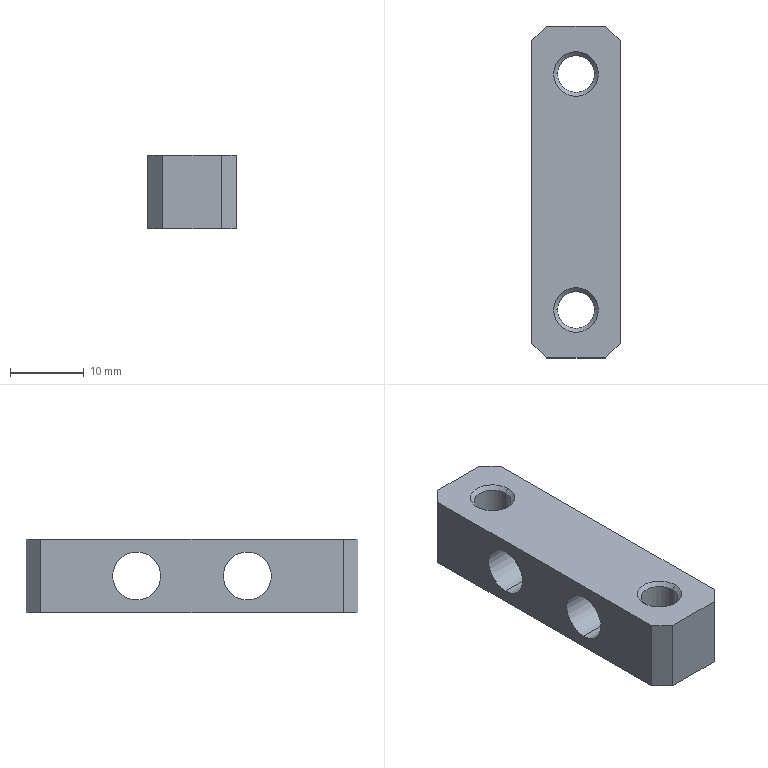Part | SolidWorks | features 3DProfileFeature 1, Chamfer 1, Extrusion 1, HoleWzd 1, ICE 1, MirrorPattern 1 | 1 solid | 22 faces | box 12 x 45 x 10 mm | volume 4126 mm3 | plane 10 | cylinder 8 | cone 4 | commonest cylinder face diameters 5 x4 6.5 x4
STEP:
#1=CARTESIAN_POINT('',(-2.5,16.,4.475));
#2=VERTEX_POINT('',#1);
#3=CARTESIAN_POINT('',(2.5,16.,4.475));
#4=VERTEX_POINT('',#3);
#5=CARTESIAN_POINT('',(0.,16.,4.475));
#6=DIRECTION('',(0.,0.,1.));
#7=DIRECTION('',(1.,0.,0.));
#8=AXIS2_PLACEMENT_3D('',#5,#6,#7);
#9=CIRCLE('',#8,2.5);
#10=EDGE_CURVE('',#2,#4,#9,.T.);
#11=ORIENTED_EDGE('',*,*,#10,.F.);
#12=CARTESIAN_POINT('',(-3.025,16.,5.));
#13=VERTEX_POINT('',#12);
#14=CARTESIAN_POINT('',(-3.025,16.,5.));
#15=DIRECTION('',(-0.7071,0.,0.7071));
#16=VECTOR('',#15,1000.);
#17=LINE('',#14,#16);
#18=EDGE_CURVE('',#2,#13,#17,.T.);
#19=ORIENTED_EDGE('',*,*,#18,.T.);
#20=CARTESIAN_POINT('',(3.025,16.,5.));
#21=VERTEX_POINT('',#20);
#22=CARTESIAN_POINT('',(0.,16.,5.));
#23=DIRECTION('',(0.,0.,1.));
#24=DIRECTION('',(1.,0.,0.));
#25=AXIS2_PLACEMENT_3D('',#22,#23,#24);
#26=CIRCLE('',#25,3.025);
#27=EDGE_CURVE('',#13,#21,#26,.T.);
#28=ORIENTED_EDGE('',*,*,#27,.T.);
#29=CARTESIAN_POINT('',(3.025,16.,5.));
#30=DIRECTION('',(0.7071,0.,0.7071));
#31=VECTOR('',#30,1000.);
#32=LINE('',#29,#31);
#33=EDGE_CURVE('',#4,#21,#32,.T.);
#34=ORIENTED_EDGE('',*,*,#33,.F.);
#35=EDGE_LOOP('',(#11,#19,#28,#34));
#36=FACE_OUTER_BOUND('',#35,.T.);
#37=CARTESIAN_POINT('',(0.,16.,5.));
#38=DIRECTION('',(0.,0.,1.));
#39=DIRECTION('',(1.,0.,0.));
#40=AXIS2_PLACEMENT_3D('',#37,#38,#39);
#41=CONICAL_SURFACE('',#40,3.025,0.7854);
#42=ADVANCED_FACE('',(#36),#41,.F.);
#43=CARTESIAN_POINT('',(2.5,16.,-5.));
#44=VERTEX_POINT('',#43);
#45=CARTESIAN_POINT('',(-2.5,16.,-5.));
#46=VERTEX_POINT('',#45);
#47=CARTESIAN_POINT('',(0.,16.,-5.));
#48=DIRECTION('',(0.,0.,-1.));
#49=DIRECTION('',(-1.,0.,0.));
#50=AXIS2_PLACEMENT_3D('',#47,#48,#49);
#51=CIRCLE('',#50,2.5);
#52=EDGE_CURVE('',#44,#46,#51,.T.);
#53=ORIENTED_EDGE('',*,*,#52,.T.);
#54=CARTESIAN_POINT('',(-2.5,16.,5.));
#55=DIRECTION('',(0.,0.,1.));
#56=VECTOR('',#55,1000.);
#57=LINE('',#54,#56);
#58=EDGE_CURVE('',#46,#2,#57,.T.);
#59=ORIENTED_EDGE('',*,*,#58,.T.);
#60=ORIENTED_EDGE('',*,*,#10,.T.);
#61=CARTESIAN_POINT('',(2.5,16.,5.));
#62=DIRECTION('',(0.,0.,1.));
#63=VECTOR('',#62,1000.);
#64=LINE('',#61,#63);
#65=EDGE_CURVE('',#44,#4,#64,.T.);
#66=ORIENTED_EDGE('',*,*,#65,.F.);
#67=EDGE_LOOP('',(#53,#59,#60,#66));
#68=FACE_OUTER_BOUND('',#67,.T.);
#69=CARTESIAN_POINT('',(0.,16.,5.));
#70=DIRECTION('',(0.,0.,1.));
#71=DIRECTION('',(1.,0.,0.));
#72=AXIS2_PLACEMENT_3D('',#69,#70,#71);
#73=CYLINDRICAL_SURFACE('',#72,2.5);
#74=ADVANCED_FACE('',(#68),#73,.F.);
#75=CARTESIAN_POINT('',(6.,7.5,3.25));
#76=VERTEX_POINT('',#75);
#77=CARTESIAN_POINT('',(6.,7.5,-3.25));
#78=VERTEX_POINT('',#77);
#79=CARTESIAN_POINT('',(6.,7.5,0.));
#80=DIRECTION('',(1.,0.,0.));
#81=DIRECTION('',(0.,0.,1.));
#82=AXIS2_PLACEMENT_3D('',#79,#80,#81);
#83=CIRCLE('',#82,3.25);
#84=EDGE_CURVE('',#76,#78,#83,.T.);
#85=ORIENTED_EDGE('',*,*,#84,.T.);
#86=CARTESIAN_POINT('',(-6.,7.5,-3.25));
#87=VERTEX_POINT('',#86);
#88=CARTESIAN_POINT('',(6.001,7.5,-3.25));
#89=DIRECTION('',(-1.,0.,0.));
#90=VECTOR('',#89,1000.);
#91=LINE('',#88,#90);
#92=EDGE_CURVE('',#78,#87,#91,.T.);
#93=ORIENTED_EDGE('',*,*,#92,.T.);
#94=CARTESIAN_POINT('',(-6.,7.5,3.25));
#95=VERTEX_POINT('',#94);
#96=CARTESIAN_POINT('',(-6.,7.5,0.));
#97=DIRECTION('',(-1.,0.,0.));
#98=DIRECTION('',(0.,0.,1.));
#99=AXIS2_PLACEMENT_3D('',#96,#97,#98);
#100=CIRCLE('',#99,3.25);
#101=EDGE_CURVE('',#87,#95,#100,.T.);
#102=ORIENTED_EDGE('',*,*,#101,.T.);
#103=CARTESIAN_POINT('',(6.001,7.5,3.25));
#104=DIRECTION('',(-1.,0.,0.));
#105=VECTOR('',#104,1000.);
#106=LINE('',#103,#105);
#107=EDGE_CURVE('',#76,#95,#106,.T.);
#108=ORIENTED_EDGE('',*,*,#107,.F.);
#109=EDGE_LOOP('',(#85,#93,#102,#108));
#110=FACE_OUTER_BOUND('',#109,.T.);
#111=CARTESIAN_POINT('',(6.001,7.5,0.));
#112=DIRECTION('',(-1.,0.,0.));
#113=DIRECTION('',(0.,0.,1.));
#114=AXIS2_PLACEMENT_3D('',#111,#112,#113);
#115=CYLINDRICAL_SURFACE('',#114,3.25);
#116=ADVANCED_FACE('',(#110),#115,.F.);
#117=CARTESIAN_POINT('',(6.,-7.5,3.25));
#118=VERTEX_POINT('',#117);
#119=CARTESIAN_POINT('',(6.,-7.5,-3.25));
#120=VERTEX_POINT('',#119);
#121=CARTESIAN_POINT('',(6.,-7.5,0.));
#122=DIRECTION('',(1.,0.,0.));
#123=DIRECTION('',(0.,0.,1.));
#124=AXIS2_PLACEMENT_3D('',#121,#122,#123);
#125=CIRCLE('',#124,3.25);
#126=EDGE_CURVE('',#118,#120,#125,.T.);
#127=ORIENTED_EDGE('',*,*,#126,.T.);
#128=CARTESIAN_POINT('',(-6.,-7.5,-3.25));
#129=VERTEX_POINT('',#128);
#130=CARTESIAN_POINT('',(6.001,-7.5,-3.25));
#131=DIRECTION('',(-1.,0.,0.));
#132=VECTOR('',#131,1000.);
#133=LINE('',#130,#132);
#134=EDGE_CURVE('',#120,#129,#133,.T.);
#135=ORIENTED_EDGE('',*,*,#134,.T.);
#136=CARTESIAN_POINT('',(-6.,-7.5,3.25));
#137=VERTEX_POINT('',#136);
#138=CARTESIAN_POINT('',(-6.,-7.5,0.));
#139=DIRECTION('',(-1.,0.,0.));
#140=DIRECTION('',(0.,0.,1.));
#141=AXIS2_PLACEMENT_3D('',#138,#139,#140);
#142=CIRCLE('',#141,3.25);
#143=EDGE_CURVE('',#129,#137,#142,.T.);
#144=ORIENTED_EDGE('',*,*,#143,.T.);
#145=CARTESIAN_POINT('',(6.001,-7.5,3.25));
#146=DIRECTION('',(-1.,0.,0.));
#147=VECTOR('',#146,1000.);
#148=LINE('',#145,#147);
#149=EDGE_CURVE('',#118,#137,#148,.T.);
#150=ORIENTED_EDGE('',*,*,#149,.F.);
#151=EDGE_LOOP('',(#127,#135,#144,#150));
#152=FACE_OUTER_BOUND('',#151,.T.);
#153=CARTESIAN_POINT('',(6.001,-7.5,0.));
#154=DIRECTION('',(-1.,0.,0.));
#155=DIRECTION('',(0.,0.,1.));
#156=AXIS2_PLACEMENT_3D('',#153,#154,#155);
#157=CYLINDRICAL_SURFACE('',#156,3.25);
#158=ADVANCED_FACE('',(#152),#157,.F.);
#159=CARTESIAN_POINT('',(-2.5,-16.,4.475));
#160=VERTEX_POINT('',#159);
#161=CARTESIAN_POINT('',(2.5,-16.,4.475));
#162=VERTEX_POINT('',#161);
#163=CARTESIAN_POINT('',(0.,-16.,4.475));
#164=DIRECTION('',(0.,0.,1.));
#165=DIRECTION('',(1.,0.,0.));
#166=AXIS2_PLACEMENT_3D('',#163,#164,#165);
#167=CIRCLE('',#166,2.5);
#168=EDGE_CURVE('',#160,#162,#167,.T.);
#169=ORIENTED_EDGE('',*,*,#168,.F.);
#170=CARTESIAN_POINT('',(-3.025,-16.,5.));
#171=VERTEX_POINT('',#170);
#172=CARTESIAN_POINT('',(-3.025,-16.,5.));
#173=DIRECTION('',(-0.7071,0.,0.7071));
#174=VECTOR('',#173,1000.);
#175=LINE('',#172,#174);
#176=EDGE_CURVE('',#160,#171,#175,.T.);
#177=ORIENTED_EDGE('',*,*,#176,.T.);
#178=CARTESIAN_POINT('',(3.025,-16.,5.));
#179=VERTEX_POINT('',#178);
#180=CARTESIAN_POINT('',(0.,-16.,5.));
#181=DIRECTION('',(0.,0.,1.));
#182=DIRECTION('',(1.,0.,0.));
#183=AXIS2_PLACEMENT_3D('',#180,#181,#182);
#184=CIRCLE('',#183,3.025);
#185=EDGE_CURVE('',#171,#179,#184,.T.);
#186=ORIENTED_EDGE('',*,*,#185,.T.);
#187=CARTESIAN_POINT('',(3.025,-16.,5.));
#188=DIRECTION('',(0.7071,0.,0.7071));
#189=VECTOR('',#188,1000.);
#190=LINE('',#187,#189);
#191=EDGE_CURVE('',#162,#179,#190,.T.);
#192=ORIENTED_EDGE('',*,*,#191,.F.);
#193=EDGE_LOOP('',(#169,#177,#186,#192));
#194=FACE_OUTER_BOUND('',#193,.T.);
#195=CARTESIAN_POINT('',(0.,-16.,5.));
#196=DIRECTION('',(0.,0.,1.));
#197=DIRECTION('',(1.,0.,0.));
#198=AXIS2_PLACEMENT_3D('',#195,#196,#197);
#199=CONICAL_SURFACE('',#198,3.025,0.7854);
#200=ADVANCED_FACE('',(#194),#199,.F.);
#201=CARTESIAN_POINT('',(2.5,-16.,-5.));
#202=VERTEX_POINT('',#201);
#203=CARTESIAN_POINT('',(-2.5,-16.,-5.));
#204=VERTEX_POINT('',#203);
#205=CARTESIAN_POINT('',(0.,-16.,-5.));
#206=DIRECTION('',(0.,0.,-1.));
#207=DIRECTION('',(-1.,0.,0.));
#208=AXIS2_PLACEMENT_3D('',#205,#206,#207);
#209=CIRCLE('',#208,2.5);
#210=EDGE_CURVE('',#202,#204,#209,.T.);
#211=ORIENTED_EDGE('',*,*,#210,.T.);
#212=CARTESIAN_POINT('',(-2.5,-16.,5.));
#213=DIRECTION('',(0.,0.,1.));
#214=VECTOR('',#213,1000.);
#215=LINE('',#212,#214);
#216=EDGE_CURVE('',#204,#160,#215,.T.);
#217=ORIENTED_EDGE('',*,*,#216,.T.);
#218=ORIENTED_EDGE('',*,*,#168,.T.);
#219=CARTESIAN_POINT('',(2.5,-16.,5.));
#220=DIRECTION('',(0.,0.,1.));
#221=VECTOR('',#220,1000.);
#222=LINE('',#219,#221);
#223=EDGE_CURVE('',#202,#162,#222,.T.);
#224=ORIENTED_EDGE('',*,*,#223,.F.);
#225=EDGE_LOOP('',(#211,#217,#218,#224));
#226=FACE_OUTER_BOUND('',#225,.T.);
#227=CARTESIAN_POINT('',(0.,-16.,5.));
#228=DIRECTION('',(0.,0.,1.));
#229=DIRECTION('',(1.,0.,0.));
#230=AXIS2_PLACEMENT_3D('',#227,#228,#229);
#231=CYLINDRICAL_SURFACE('',#230,2.5);
#232=ADVANCED_FACE('',(#226),#231,.F.);
#233=CARTESIAN_POINT('',(4.,22.5,5.));
#234=VERTEX_POINT('',#233);
#235=CARTESIAN_POINT('',(-4.,22.5,5.));
#236=VERTEX_POINT('',#235);
#237=CARTESIAN_POINT('',(-6.,22.5,5.));
#238=DIRECTION('',(-1.,0.,0.));
#239=VECTOR('',#238,1000.);
#240=LINE('',#237,#239);
#241=EDGE_CURVE('',#234,#236,#240,.T.);
#242=ORIENTED_EDGE('',*,*,#241,.T.);
#243=CARTESIAN_POINT('',(-6.,20.5,5.));
#244=VERTEX_POINT('',#243);
#245=CARTESIAN_POINT('',(-6.,20.5,5.));
#246=DIRECTION('',(-0.7071,-0.7071,0.));
#247=VECTOR('',#246,1000.);
#248=LINE('',#245,#247);
#249=EDGE_CURVE('',#236,#244,#248,.T.);
#250=ORIENTED_EDGE('',*,*,#249,.T.);
#251=CARTESIAN_POINT('',(-6.,-20.5,5.));
#252=VERTEX_POINT('',#251);
#253=CARTESIAN_POINT('',(-6.,-22.5,5.));
#254=DIRECTION('',(0.,-1.,0.));
#255=VECTOR('',#254,1000.);
#256=LINE('',#253,#255);
#257=EDGE_CURVE('',#244,#252,#256,.T.);
#258=ORIENTED_EDGE('',*,*,#257,.T.);
#259=CARTESIAN_POINT('',(-4.,-22.5,5.));
#260=VERTEX_POINT('',#259);
#261=CARTESIAN_POINT('',(-4.,-22.5,5.));
#262=DIRECTION('',(0.7071,-0.7071,0.));
#263=VECTOR('',#262,1000.);
#264=LINE('',#261,#263);
#265=EDGE_CURVE('',#252,#260,#264,.T.);
#266=ORIENTED_EDGE('',*,*,#265,.T.);
#267=CARTESIAN_POINT('',(4.,-22.5,5.));
#268=VERTEX_POINT('',#267);
#269=CARTESIAN_POINT('',(-6.,-22.5,5.));
#270=DIRECTION('',(1.,0.,0.));
#271=VECTOR('',#270,1000.);
#272=LINE('',#269,#271);
#273=EDGE_CURVE('',#260,#268,#272,.T.);
#274=ORIENTED_EDGE('',*,*,#273,.T.);
#275=CARTESIAN_POINT('',(6.,-20.5,5.));
#276=VERTEX_POINT('',#275);
#277=CARTESIAN_POINT('',(6.,-20.5,5.));
#278=DIRECTION('',(0.7071,0.7071,0.));
#279=VECTOR('',#278,1000.);
#280=LINE('',#277,#279);
#281=EDGE_CURVE('',#268,#276,#280,.T.);
#282=ORIENTED_EDGE('',*,*,#281,.T.);
#283=CARTESIAN_POINT('',(6.,20.5,5.));
#284=VERTEX_POINT('',#283);
#285=CARTESIAN_POINT('',(6.,-22.5,5.));
#286=DIRECTION('',(0.,1.,0.));
#287=VECTOR('',#286,1000.);
#288=LINE('',#285,#287);
#289=EDGE_CURVE('',#276,#284,#288,.T.);
#290=ORIENTED_EDGE('',*,*,#289,.T.);
#291=CARTESIAN_POINT('',(4.,22.5,5.));
#292=DIRECTION('',(-0.7071,0.7071,0.));
#293=VECTOR('',#292,1000.);
#294=LINE('',#291,#293);
#295=EDGE_CURVE('',#284,#234,#294,.T.);
#296=ORIENTED_EDGE('',*,*,#295,.T.);
#297=EDGE_LOOP('',(#242,#250,#258,#266,#274,#282,#290,#296));
#298=FACE_OUTER_BOUND('',#297,.T.);
#299=CARTESIAN_POINT('',(0.,-16.,5.));
#300=DIRECTION('',(0.,0.,1.));
#301=DIRECTION('',(1.,0.,0.));
#302=AXIS2_PLACEMENT_3D('',#299,#300,#301);
#303=CIRCLE('',#302,3.025);
#304=EDGE_CURVE('',#179,#171,#303,.T.);
#305=ORIENTED_EDGE('',*,*,#304,.F.);
#306=ORIENTED_EDGE('',*,*,#185,.F.);
#307=EDGE_LOOP('',(#305,#306));
#308=FACE_BOUND('',#307,.T.);
#309=CARTESIAN_POINT('',(0.,16.,5.));
#310=DIRECTION('',(0.,0.,1.));
#311=DIRECTION('',(1.,0.,0.));
#312=AXIS2_PLACEMENT_3D('',#309,#310,#311);
#313=CIRCLE('',#312,3.025);
#314=EDGE_CURVE('',#21,#13,#313,.T.);
#315=ORIENTED_EDGE('',*,*,#314,.F.);
#316=ORIENTED_EDGE('',*,*,#27,.F.);
#317=EDGE_LOOP('',(#315,#316));
#318=FACE_BOUND('',#317,.T.);
#319=CARTESIAN_POINT('',(0.,0.,5.));
#320=DIRECTION('',(0.,0.,-1.));
#321=DIRECTION('',(-1.,0.,0.));
#322=AXIS2_PLACEMENT_3D('',#319,#320,#321);
#323=PLANE('',#322);
#324=ADVANCED_FACE('',(#298,#308,#318),#323,.F.);
#325=ORIENTED_EDGE('',*,*,#84,.F.);
#326=CARTESIAN_POINT('',(6.,7.5,0.));
#327=DIRECTION('',(1.,0.,0.));
#328=DIRECTION('',(0.,0.,1.));
#329=AXIS2_PLACEMENT_3D('',#326,#327,#328);
#330=CIRCLE('',#329,3.25);
#331=EDGE_CURVE('',#78,#76,#330,.T.);
#332=ORIENTED_EDGE('',*,*,#331,.F.);
#333=EDGE_LOOP('',(#325,#332));
#334=FACE_BOUND('',#333,.T.);
#335=ORIENTED_EDGE('',*,*,#126,.F.);
#336=CARTESIAN_POINT('',(6.,-7.5,0.));
#337=DIRECTION('',(1.,0.,0.));
#338=DIRECTION('',(0.,0.,1.));
#339=AXIS2_PLACEMENT_3D('',#336,#337,#338);
#340=CIRCLE('',#339,3.25);
#341=EDGE_CURVE('',#120,#118,#340,.T.);
#342=ORIENTED_EDGE('',*,*,#341,.F.);
#343=EDGE_LOOP('',(#335,#342));
#344=FACE_BOUND('',#343,.T.);
#345=CARTESIAN_POINT('',(6.,-20.5,-5.));
#346=VERTEX_POINT('',#345);
#347=CARTESIAN_POINT('',(6.,20.5,-5.));
#348=VERTEX_POINT('',#347);
#349=CARTESIAN_POINT('',(6.,-22.5,-5.));
#350=DIRECTION('',(0.,1.,0.));
#351=VECTOR('',#350,1000.);
#352=LINE('',#349,#351);
#353=EDGE_CURVE('',#346,#348,#352,.T.);
#354=ORIENTED_EDGE('',*,*,#353,.T.);
#355=CARTESIAN_POINT('',(6.,20.5,5.));
#356=DIRECTION('',(0.,0.,1.));
#357=VECTOR('',#356,1000.);
#358=LINE('',#355,#357);
#359=EDGE_CURVE('',#348,#284,#358,.T.);
#360=ORIENTED_EDGE('',*,*,#359,.T.);
#361=ORIENTED_EDGE('',*,*,#289,.F.);
#362=CARTESIAN_POINT('',(6.,-20.5,5.));
#363=DIRECTION('',(0.,0.,-1.));
#364=VECTOR('',#363,1000.);
#365=LINE('',#362,#364);
#366=EDGE_CURVE('',#276,#346,#365,.T.);
#367=ORIENTED_EDGE('',*,*,#366,.T.);
#368=EDGE_LOOP('',(#354,#360,#361,#367));
#369=FACE_OUTER_BOUND('',#368,.T.);
#370=CARTESIAN_POINT('',(6.,-22.5,5.));
#371=DIRECTION('',(-1.,0.,0.));
#372=DIRECTION('',(0.,0.,1.));
#373=AXIS2_PLACEMENT_3D('',#370,#371,#372);
#374=PLANE('',#373);
#375=ADVANCED_FACE('',(#334,#344,#369),#374,.F.);
#376=CARTESIAN_POINT('',(4.,22.5,-5.));
#377=VERTEX_POINT('',#376);
#378=CARTESIAN_POINT('',(-4.,22.5,-5.));
#379=VERTEX_POINT('',#378);
#380=CARTESIAN_POINT('',(-6.,22.5,-5.));
#381=DIRECTION('',(-1.,0.,0.));
#382=VECTOR('',#381,1000.);
#383=LINE('',#380,#382);
#384=EDGE_CURVE('',#377,#379,#383,.T.);
#385=ORIENTED_EDGE('',*,*,#384,.T.);
#386=CARTESIAN_POINT('',(-4.,22.5,5.));
#387=DIRECTION('',(0.,0.,1.));
#388=VECTOR('',#387,1000.);
#389=LINE('',#386,#388);
#390=EDGE_CURVE('',#379,#236,#389,.T.);
#391=ORIENTED_EDGE('',*,*,#390,.T.);
#392=ORIENTED_EDGE('',*,*,#241,.F.);
#393=CARTESIAN_POINT('',(4.,22.5,5.));
#394=DIRECTION('',(0.,0.,-1.));
#395=VECTOR('',#394,1000.);
#396=LINE('',#393,#395);
#397=EDGE_CURVE('',#234,#377,#396,.T.);
#398=ORIENTED_EDGE('',*,*,#397,.T.);
#399=EDGE_LOOP('',(#385,#391,#392,#398));
#400=FACE_OUTER_BOUND('',#399,.T.);
#401=CARTESIAN_POINT('',(-6.,22.5,5.));
#402=DIRECTION('',(0.,-1.,0.));
#403=DIRECTION('',(0.,0.,-1.));
#404=AXIS2_PLACEMENT_3D('',#401,#402,#403);
#405=PLANE('',#404);
#406=ADVANCED_FACE('',(#400),#405,.F.);
#407=CARTESIAN_POINT('',(-6.,7.5,0.));
#408=DIRECTION('',(-1.,0.,0.));
#409=DIRECTION('',(0.,0.,1.));
#410=AXIS2_PLACEMENT_3D('',#407,#408,#409);
#411=CIRCLE('',#410,3.25);
#412=EDGE_CURVE('',#95,#87,#411,.T.);
#413=ORIENTED_EDGE('',*,*,#412,.F.);
#414=ORIENTED_EDGE('',*,*,#101,.F.);
#415=EDGE_LOOP('',(#413,#414));
#416=FACE_BOUND('',#415,.T.);
#417=CARTESIAN_POINT('',(-6.,-7.5,0.));
#418=DIRECTION('',(-1.,0.,0.));
#419=DIRECTION('',(0.,0.,1.));
#420=AXIS2_PLACEMENT_3D('',#417,#418,#419);
#421=CIRCLE('',#420,3.25);
#422=EDGE_CURVE('',#137,#129,#421,.T.);
#423=ORIENTED_EDGE('',*,*,#422,.F.);
#424=ORIENTED_EDGE('',*,*,#143,.F.);
#425=EDGE_LOOP('',(#423,#424));
#426=FACE_BOUND('',#425,.T.);
#427=ORIENTED_EDGE('',*,*,#257,.F.);
#428=CARTESIAN_POINT('',(-6.,20.5,-5.));
#429=VERTEX_POINT('',#428);
#430=CARTESIAN_POINT('',(-6.,20.5,5.));
#431=DIRECTION('',(0.,0.,-1.));
#432=VECTOR('',#431,1000.);
#433=LINE('',#430,#432);
#434=EDGE_CURVE('',#244,#429,#433,.T.);
#435=ORIENTED_EDGE('',*,*,#434,.T.);
#436=CARTESIAN_POINT('',(-6.,-20.5,-5.));
#437=VERTEX_POINT('',#436);
#438=CARTESIAN_POINT('',(-6.,-22.5,-5.));
#439=DIRECTION('',(0.,-1.,0.));
#440=VECTOR('',#439,1000.);
#441=LINE('',#438,#440);
#442=EDGE_CURVE('',#429,#437,#441,.T.);
#443=ORIENTED_EDGE('',*,*,#442,.T.);
#444=CARTESIAN_POINT('',(-6.,-20.5,5.));
#445=DIRECTION('',(0.,0.,1.));
#446=VECTOR('',#445,1000.);
#447=LINE('',#444,#446);
#448=EDGE_CURVE('',#437,#252,#447,.T.);
#449=ORIENTED_EDGE('',*,*,#448,.T.);
#450=EDGE_LOOP('',(#427,#435,#443,#449));
#451=FACE_OUTER_BOUND('',#450,.T.);
#452=CARTESIAN_POINT('',(-6.,-22.5,5.));
#453=DIRECTION('',(1.,0.,0.));
#454=DIRECTION('',(0.,0.,-1.));
#455=AXIS2_PLACEMENT_3D('',#452,#453,#454);
#456=PLANE('',#455);
#457=ADVANCED_FACE('',(#416,#426,#451),#456,.F.);
#458=ORIENTED_EDGE('',*,*,#273,.F.);
#459=CARTESIAN_POINT('',(-4.,-22.5,-5.));
#460=VERTEX_POINT('',#459);
#461=CARTESIAN_POINT('',(-4.,-22.5,5.));
#462=DIRECTION('',(0.,0.,-1.));
#463=VECTOR('',#462,1000.);
#464=LINE('',#461,#463);
#465=EDGE_CURVE('',#260,#460,#464,.T.);
#466=ORIENTED_EDGE('',*,*,#465,.T.);
#467=CARTESIAN_POINT('',(4.,-22.5,-5.));
#468=VERTEX_POINT('',#467);
#469=CARTESIAN_POINT('',(-6.,-22.5,-5.));
#470=DIRECTION('',(1.,0.,0.));
#471=VECTOR('',#470,1000.);
#472=LINE('',#469,#471);
#473=EDGE_CURVE('',#460,#468,#472,.T.);
#474=ORIENTED_EDGE('',*,*,#473,.T.);
#475=CARTESIAN_POINT('',(4.,-22.5,5.));
#476=DIRECTION('',(0.,0.,1.));
#477=VECTOR('',#476,1000.);
#478=LINE('',#475,#477);
#479=EDGE_CURVE('',#468,#268,#478,.T.);
#480=ORIENTED_EDGE('',*,*,#479,.T.);
#481=EDGE_LOOP('',(#458,#466,#474,#480));
#482=FACE_OUTER_BOUND('',#481,.T.);
#483=CARTESIAN_POINT('',(-6.,-22.5,5.));
#484=DIRECTION('',(0.,1.,0.));
#485=DIRECTION('',(0.,0.,1.));
#486=AXIS2_PLACEMENT_3D('',#483,#484,#485);
#487=PLANE('',#486);
#488=ADVANCED_FACE('',(#482),#487,.F.);
#489=ORIENTED_EDGE('',*,*,#52,.F.);
#490=CARTESIAN_POINT('',(0.,16.,-5.));
#491=DIRECTION('',(0.,0.,-1.));
#492=DIRECTION('',(-1.,0.,0.));
#493=AXIS2_PLACEMENT_3D('',#490,#491,#492);
#494=CIRCLE('',#493,2.5);
#495=EDGE_CURVE('',#46,#44,#494,.T.);
#496=ORIENTED_EDGE('',*,*,#495,.F.);
#497=EDGE_LOOP('',(#489,#496));
#498=FACE_BOUND('',#497,.T.);
#499=ORIENTED_EDGE('',*,*,#210,.F.);
#500=CARTESIAN_POINT('',(0.,-16.,-5.));
#501=DIRECTION('',(0.,0.,-1.));
#502=DIRECTION('',(-1.,0.,0.));
#503=AXIS2_PLACEMENT_3D('',#500,#501,#502);
#504=CIRCLE('',#503,2.5);
#505=EDGE_CURVE('',#204,#202,#504,.T.);
#506=ORIENTED_EDGE('',*,*,#505,.F.);
#507=EDGE_LOOP('',(#499,#506));
#508=FACE_BOUND('',#507,.T.);
#509=ORIENTED_EDGE('',*,*,#442,.F.);
#510=CARTESIAN_POINT('',(-13.25,13.25,-5.));
#511=DIRECTION('',(0.7071,0.7071,0.));
#512=VECTOR('',#511,1000.);
#513=LINE('',#510,#512);
#514=EDGE_CURVE('',#429,#379,#513,.T.);
#515=ORIENTED_EDGE('',*,*,#514,.T.);
#516=ORIENTED_EDGE('',*,*,#384,.F.);
#517=CARTESIAN_POINT('',(13.25,13.25,-5.));
#518=DIRECTION('',(0.7071,-0.7071,0.));
#519=VECTOR('',#518,1000.);
#520=LINE('',#517,#519);
#521=EDGE_CURVE('',#377,#348,#520,.T.);
#522=ORIENTED_EDGE('',*,*,#521,.T.);
#523=ORIENTED_EDGE('',*,*,#353,.F.);
#524=CARTESIAN_POINT('',(13.25,-13.25,-5.));
#525=DIRECTION('',(-0.7071,-0.7071,0.));
#526=VECTOR('',#525,1000.);
#527=LINE('',#524,#526);
#528=EDGE_CURVE('',#346,#468,#527,.T.);
#529=ORIENTED_EDGE('',*,*,#528,.T.);
#530=ORIENTED_EDGE('',*,*,#473,.F.);
#531=CARTESIAN_POINT('',(-13.25,-13.25,-5.));
#532=DIRECTION('',(-0.7071,0.7071,0.));
#533=VECTOR('',#532,1000.);
#534=LINE('',#531,#533);
#535=EDGE_CURVE('',#460,#437,#534,.T.);
#536=ORIENTED_EDGE('',*,*,#535,.T.);
#537=EDGE_LOOP('',(#509,#515,#516,#522,#523,#529,#530,#536));
#538=FACE_OUTER_BOUND('',#537,.T.);
#539=CARTESIAN_POINT('',(0.,0.,-5.));
#540=DIRECTION('',(0.,0.,-1.));
#541=DIRECTION('',(-1.,0.,0.));
#542=AXIS2_PLACEMENT_3D('',#539,#540,#541);
#543=PLANE('',#542);
#544=ADVANCED_FACE('',(#498,#508,#538),#543,.T.);
#545=ORIENTED_EDGE('',*,*,#216,.F.);
#546=ORIENTED_EDGE('',*,*,#505,.T.);
#547=ORIENTED_EDGE('',*,*,#223,.T.);
#548=CARTESIAN_POINT('',(0.,-16.,4.475));
#549=DIRECTION('',(0.,0.,1.));
#550=DIRECTION('',(1.,0.,0.));
#551=AXIS2_PLACEMENT_3D('',#548,#549,#550);
#552=CIRCLE('',#551,2.5);
#553=EDGE_CURVE('',#162,#160,#552,.T.);
#554=ORIENTED_EDGE('',*,*,#553,.T.);
#555=EDGE_LOOP('',(#545,#546,#547,#554));
#556=FACE_OUTER_BOUND('',#555,.T.);
#557=CARTESIAN_POINT('',(0.,-16.,5.));
#558=DIRECTION('',(0.,0.,1.));
#559=DIRECTION('',(1.,0.,0.));
#560=AXIS2_PLACEMENT_3D('',#557,#558,#559);
#561=CYLINDRICAL_SURFACE('',#560,2.5);
#562=ADVANCED_FACE('',(#556),#561,.F.);
#563=ORIENTED_EDGE('',*,*,#176,.F.);
#564=ORIENTED_EDGE('',*,*,#553,.F.);
#565=ORIENTED_EDGE('',*,*,#191,.T.);
#566=ORIENTED_EDGE('',*,*,#304,.T.);
#567=EDGE_LOOP('',(#563,#564,#565,#566));
#568=FACE_OUTER_BOUND('',#567,.T.);
#569=CARTESIAN_POINT('',(0.,-16.,5.));
#570=DIRECTION('',(0.,0.,1.));
#571=DIRECTION('',(1.,0.,0.));
#572=AXIS2_PLACEMENT_3D('',#569,#570,#571);
#573=CONICAL_SURFACE('',#572,3.025,0.7854);
#574=ADVANCED_FACE('',(#568),#573,.F.);
#575=ORIENTED_EDGE('',*,*,#134,.F.);
#576=ORIENTED_EDGE('',*,*,#341,.T.);
#577=ORIENTED_EDGE('',*,*,#149,.T.);
#578=ORIENTED_EDGE('',*,*,#422,.T.);
#579=EDGE_LOOP('',(#575,#576,#577,#578));
#580=FACE_OUTER_BOUND('',#579,.T.);
#581=CARTESIAN_POINT('',(6.001,-7.5,0.));
#582=DIRECTION('',(-1.,0.,0.));
#583=DIRECTION('',(0.,0.,1.));
#584=AXIS2_PLACEMENT_3D('',#581,#582,#583);
#585=CYLINDRICAL_SURFACE('',#584,3.25);
#586=ADVANCED_FACE('',(#580),#585,.F.);
#587=ORIENTED_EDGE('',*,*,#92,.F.);
#588=ORIENTED_EDGE('',*,*,#331,.T.);
#589=ORIENTED_EDGE('',*,*,#107,.T.);
#590=ORIENTED_EDGE('',*,*,#412,.T.);
#591=EDGE_LOOP('',(#587,#588,#589,#590));
#592=FACE_OUTER_BOUND('',#591,.T.);
#593=CARTESIAN_POINT('',(6.001,7.5,0.));
#594=DIRECTION('',(-1.,0.,0.));
#595=DIRECTION('',(0.,0.,1.));
#596=AXIS2_PLACEMENT_3D('',#593,#594,#595);
#597=CYLINDRICAL_SURFACE('',#596,3.25);
#598=ADVANCED_FACE('',(#592),#597,.F.);
#599=ORIENTED_EDGE('',*,*,#58,.F.);
#600=ORIENTED_EDGE('',*,*,#495,.T.);
#601=ORIENTED_EDGE('',*,*,#65,.T.);
#602=CARTESIAN_POINT('',(0.,16.,4.475));
#603=DIRECTION('',(0.,0.,1.));
#604=DIRECTION('',(1.,0.,0.));
#605=AXIS2_PLACEMENT_3D('',#602,#603,#604);
#606=CIRCLE('',#605,2.5);
#607=EDGE_CURVE('',#4,#2,#606,.T.);
#608=ORIENTED_EDGE('',*,*,#607,.T.);
#609=EDGE_LOOP('',(#599,#600,#601,#608));
#610=FACE_OUTER_BOUND('',#609,.T.);
#611=CARTESIAN_POINT('',(0.,16.,5.));
#612=DIRECTION('',(0.,0.,1.));
#613=DIRECTION('',(1.,0.,0.));
#614=AXIS2_PLACEMENT_3D('',#611,#612,#613);
#615=CYLINDRICAL_SURFACE('',#614,2.5);
#616=ADVANCED_FACE('',(#610),#615,.F.);
#617=ORIENTED_EDGE('',*,*,#18,.F.);
#618=ORIENTED_EDGE('',*,*,#607,.F.);
#619=ORIENTED_EDGE('',*,*,#33,.T.);
#620=ORIENTED_EDGE('',*,*,#314,.T.);
#621=EDGE_LOOP('',(#617,#618,#619,#620));
#622=FACE_OUTER_BOUND('',#621,.T.);
#623=CARTESIAN_POINT('',(0.,16.,5.));
#624=DIRECTION('',(0.,0.,1.));
#625=DIRECTION('',(1.,0.,0.));
#626=AXIS2_PLACEMENT_3D('',#623,#624,#625);
#627=CONICAL_SURFACE('',#626,3.025,0.7854);
#628=ADVANCED_FACE('',(#622),#627,.F.);
#629=ORIENTED_EDGE('',*,*,#249,.F.);
#630=ORIENTED_EDGE('',*,*,#390,.F.);
#631=ORIENTED_EDGE('',*,*,#514,.F.);
#632=ORIENTED_EDGE('',*,*,#434,.F.);
#633=EDGE_LOOP('',(#629,#630,#631,#632));
#634=FACE_OUTER_BOUND('',#633,.T.);
#635=CARTESIAN_POINT('',(-6.,20.5,5.));
#636=DIRECTION('',(0.7071,-0.7071,0.));
#637=DIRECTION('',(0.,0.,-1.));
#638=AXIS2_PLACEMENT_3D('',#635,#636,#637);
#639=PLANE('',#638);
#640=ADVANCED_FACE('',(#634),#639,.F.);
#641=ORIENTED_EDGE('',*,*,#295,.F.);
#642=ORIENTED_EDGE('',*,*,#359,.F.);
#643=ORIENTED_EDGE('',*,*,#521,.F.);
#644=ORIENTED_EDGE('',*,*,#397,.F.);
#645=EDGE_LOOP('',(#641,#642,#643,#644));
#646=FACE_OUTER_BOUND('',#645,.T.);
#647=CARTESIAN_POINT('',(4.,22.5,5.));
#648=DIRECTION('',(-0.7071,-0.7071,0.));
#649=DIRECTION('',(0.,0.,-1.));
#650=AXIS2_PLACEMENT_3D('',#647,#648,#649);
#651=PLANE('',#650);
#652=ADVANCED_FACE('',(#646),#651,.F.);
#653=ORIENTED_EDGE('',*,*,#265,.F.);
#654=ORIENTED_EDGE('',*,*,#448,.F.);
#655=ORIENTED_EDGE('',*,*,#535,.F.);
#656=ORIENTED_EDGE('',*,*,#465,.F.);
#657=EDGE_LOOP('',(#653,#654,#655,#656));
#658=FACE_OUTER_BOUND('',#657,.T.);
#659=CARTESIAN_POINT('',(-4.,-22.5,5.));
#660=DIRECTION('',(0.7071,0.7071,0.));
#661=DIRECTION('',(0.,0.,-1.));
#662=AXIS2_PLACEMENT_3D('',#659,#660,#661);
#663=PLANE('',#662);
#664=ADVANCED_FACE('',(#658),#663,.F.);
#665=ORIENTED_EDGE('',*,*,#281,.F.);
#666=ORIENTED_EDGE('',*,*,#479,.F.);
#667=ORIENTED_EDGE('',*,*,#528,.F.);
#668=ORIENTED_EDGE('',*,*,#366,.F.);
#669=EDGE_LOOP('',(#665,#666,#667,#668));
#670=FACE_OUTER_BOUND('',#669,.T.);
#671=CARTESIAN_POINT('',(6.,-20.5,5.));
#672=DIRECTION('',(-0.7071,0.7071,0.));
#673=DIRECTION('',(0.,0.,-1.));
#674=AXIS2_PLACEMENT_3D('',#671,#672,#673);
#675=PLANE('',#674);
#676=ADVANCED_FACE('',(#670),#675,.F.);
#677=CLOSED_SHELL('',(#42,#74,#116,#158,#200,#232,#324,#375,#406,#457,#488,#544,#562,#574,#586,#598,#616,#628,#640,#652,#664,#676));
#678=MANIFOLD_SOLID_BREP('',#677);
#679=CARTESIAN_POINT('',(0.,0.,0.));
#680=DIRECTION('',(0.,0.,1.));
#681=DIRECTION('',(1.,0.,0.));
#682=AXIS2_PLACEMENT_3D('',#679,#680,#681);
#683=(LENGTH_UNIT()NAMED_UNIT(*)SI_UNIT(.MILLI.,.METRE.));
#684=UNCERTAINTY_MEASURE_WITH_UNIT(LENGTH_MEASURE(0.00001),#683,'','');
#685=(NAMED_UNIT(*)PLANE_ANGLE_UNIT()SI_UNIT($,.RADIAN.));
#686=(NAMED_UNIT(*)SI_UNIT($,.STERADIAN.)SOLID_ANGLE_UNIT());
#687=(GEOMETRIC_REPRESENTATION_CONTEXT(3)GLOBAL_UNCERTAINTY_ASSIGNED_CONTEXT((#684))GLOBAL_UNIT_ASSIGNED_CONTEXT((#683,#685,#686))REPRESENTATION_CONTEXT('',''));
#688=ADVANCED_BREP_SHAPE_REPRESENTATION('',(#678,#682),#687);